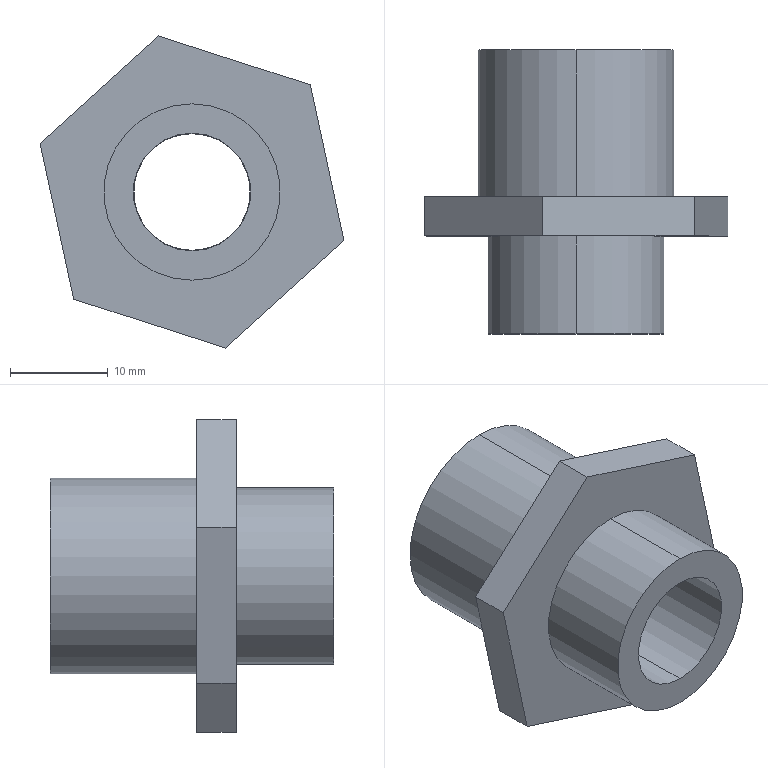Part | SolidWorks | features ICE 2, Extrusion 1 | 2 solids | 19 faces | box 31.039 x 29 x 31.865 mm | volume 6770 mm3 | plane 11 | cylinder 8 | commonest cylinder face diameters 11.911 x2 12 x2 18 x2 20 x2
STEP:
#1=CARTESIAN_POINT('',(0.,10.,-6.));
#2=VERTEX_POINT('',#1);
#3=CARTESIAN_POINT('',(0.,10.,6.));
#4=VERTEX_POINT('',#3);
#5=CARTESIAN_POINT('',(0.,10.,0.));
#6=DIRECTION('',(0.,1.,0.));
#7=DIRECTION('',(0.,0.,1.));
#8=AXIS2_PLACEMENT_3D('',#5,#6,#7);
#9=CIRCLE('',#8,6.);
#10=EDGE_CURVE('',#2,#4,#9,.T.);
#11=ORIENTED_EDGE('',*,*,#10,.T.);
#12=CARTESIAN_POINT('',(0.,0.,6.));
#13=VERTEX_POINT('',#12);
#14=CARTESIAN_POINT('',(0.,10.,6.));
#15=DIRECTION('',(0.,-1.,0.));
#16=VECTOR('',#15,1000.);
#17=LINE('',#14,#16);
#18=EDGE_CURVE('',#4,#13,#17,.T.);
#19=ORIENTED_EDGE('',*,*,#18,.T.);
#20=CARTESIAN_POINT('',(0.,0.,-6.));
#21=VERTEX_POINT('',#20);
#22=CARTESIAN_POINT('',(0.,0.,0.));
#23=DIRECTION('',(0.,1.,0.));
#24=DIRECTION('',(0.,0.,1.));
#25=AXIS2_PLACEMENT_3D('',#22,#23,#24);
#26=CIRCLE('',#25,6.);
#27=EDGE_CURVE('',#21,#13,#26,.T.);
#28=ORIENTED_EDGE('',*,*,#27,.F.);
#29=CARTESIAN_POINT('',(0.,10.,-6.));
#30=DIRECTION('',(0.,-1.,0.));
#31=VECTOR('',#30,1000.);
#32=LINE('',#29,#31);
#33=EDGE_CURVE('',#2,#21,#32,.T.);
#34=ORIENTED_EDGE('',*,*,#33,.F.);
#35=EDGE_LOOP('',(#11,#19,#28,#34));
#36=FACE_OUTER_BOUND('',#35,.T.);
#37=CARTESIAN_POINT('',(0.,10.,0.));
#38=DIRECTION('',(0.,-1.,0.));
#39=DIRECTION('',(0.,0.,-1.));
#40=AXIS2_PLACEMENT_3D('',#37,#38,#39);
#41=CYLINDRICAL_SURFACE('',#40,6.);
#42=ADVANCED_FACE('',(#36),#41,.F.);
#43=CARTESIAN_POINT('',(0.,10.,9.));
#44=VERTEX_POINT('',#43);
#45=CARTESIAN_POINT('',(0.,10.,-9.));
#46=VERTEX_POINT('',#45);
#47=CARTESIAN_POINT('',(0.,10.,0.));
#48=DIRECTION('',(0.,1.,0.));
#49=DIRECTION('',(0.,0.,1.));
#50=AXIS2_PLACEMENT_3D('',#47,#48,#49);
#51=CIRCLE('',#50,9.);
#52=EDGE_CURVE('',#44,#46,#51,.T.);
#53=ORIENTED_EDGE('',*,*,#52,.F.);
#54=CARTESIAN_POINT('',(0.,0.,9.));
#55=VERTEX_POINT('',#54);
#56=CARTESIAN_POINT('',(0.,10.,9.));
#57=DIRECTION('',(0.,-1.,0.));
#58=VECTOR('',#57,1000.);
#59=LINE('',#56,#58);
#60=EDGE_CURVE('',#44,#55,#59,.T.);
#61=ORIENTED_EDGE('',*,*,#60,.T.);
#62=CARTESIAN_POINT('',(0.,0.,-9.));
#63=VERTEX_POINT('',#62);
#64=CARTESIAN_POINT('',(0.,0.,0.));
#65=DIRECTION('',(0.,1.,0.));
#66=DIRECTION('',(0.,0.,1.));
#67=AXIS2_PLACEMENT_3D('',#64,#65,#66);
#68=CIRCLE('',#67,9.);
#69=EDGE_CURVE('',#55,#63,#68,.T.);
#70=ORIENTED_EDGE('',*,*,#69,.T.);
#71=CARTESIAN_POINT('',(0.,10.,-9.));
#72=DIRECTION('',(0.,-1.,0.));
#73=VECTOR('',#72,1000.);
#74=LINE('',#71,#73);
#75=EDGE_CURVE('',#46,#63,#74,.T.);
#76=ORIENTED_EDGE('',*,*,#75,.F.);
#77=EDGE_LOOP('',(#53,#61,#70,#76));
#78=FACE_OUTER_BOUND('',#77,.T.);
#79=CARTESIAN_POINT('',(0.,10.,0.));
#80=DIRECTION('',(0.,-1.,0.));
#81=DIRECTION('',(0.,0.,-1.));
#82=AXIS2_PLACEMENT_3D('',#79,#80,#81);
#83=CYLINDRICAL_SURFACE('',#82,9.);
#84=ADVANCED_FACE('',(#78),#83,.T.);
#85=CARTESIAN_POINT('',(0.,10.,0.));
#86=DIRECTION('',(0.,1.,0.));
#87=DIRECTION('',(0.,0.,1.));
#88=AXIS2_PLACEMENT_3D('',#85,#86,#87);
#89=CIRCLE('',#88,9.);
#90=EDGE_CURVE('',#46,#44,#89,.T.);
#91=ORIENTED_EDGE('',*,*,#90,.T.);
#92=ORIENTED_EDGE('',*,*,#52,.T.);
#93=EDGE_LOOP('',(#91,#92));
#94=FACE_OUTER_BOUND('',#93,.T.);
#95=ORIENTED_EDGE('',*,*,#10,.F.);
#96=CARTESIAN_POINT('',(0.,10.,0.));
#97=DIRECTION('',(0.,1.,0.));
#98=DIRECTION('',(0.,0.,1.));
#99=AXIS2_PLACEMENT_3D('',#96,#97,#98);
#100=CIRCLE('',#99,6.);
#101=EDGE_CURVE('',#4,#2,#100,.T.);
#102=ORIENTED_EDGE('',*,*,#101,.F.);
#103=EDGE_LOOP('',(#95,#102));
#104=FACE_BOUND('',#103,.T.);
#105=CARTESIAN_POINT('',(0.,10.,0.));
#106=DIRECTION('',(0.,1.,0.));
#107=DIRECTION('',(0.,0.,1.));
#108=AXIS2_PLACEMENT_3D('',#105,#106,#107);
#109=PLANE('',#108);
#110=ADVANCED_FACE('',(#94,#104),#109,.T.);
#111=CARTESIAN_POINT('',(0.,0.,0.));
#112=DIRECTION('',(0.,1.,0.));
#113=DIRECTION('',(0.,0.,1.));
#114=AXIS2_PLACEMENT_3D('',#111,#112,#113);
#115=CIRCLE('',#114,9.);
#116=EDGE_CURVE('',#63,#55,#115,.T.);
#117=ORIENTED_EDGE('',*,*,#116,.F.);
#118=ORIENTED_EDGE('',*,*,#69,.F.);
#119=EDGE_LOOP('',(#117,#118));
#120=FACE_OUTER_BOUND('',#119,.T.);
#121=ORIENTED_EDGE('',*,*,#27,.T.);
#122=CARTESIAN_POINT('',(0.,0.,0.));
#123=DIRECTION('',(0.,1.,0.));
#124=DIRECTION('',(0.,0.,1.));
#125=AXIS2_PLACEMENT_3D('',#122,#123,#124);
#126=CIRCLE('',#125,6.);
#127=EDGE_CURVE('',#13,#21,#126,.T.);
#128=ORIENTED_EDGE('',*,*,#127,.T.);
#129=EDGE_LOOP('',(#121,#128));
#130=FACE_BOUND('',#129,.T.);
#131=CARTESIAN_POINT('',(0.,0.,0.));
#132=DIRECTION('',(0.,1.,0.));
#133=DIRECTION('',(0.,0.,1.));
#134=AXIS2_PLACEMENT_3D('',#131,#132,#133);
#135=PLANE('',#134);
#136=ADVANCED_FACE('',(#120,#130),#135,.F.);
#137=ORIENTED_EDGE('',*,*,#60,.F.);
#138=ORIENTED_EDGE('',*,*,#90,.F.);
#139=ORIENTED_EDGE('',*,*,#75,.T.);
#140=ORIENTED_EDGE('',*,*,#116,.T.);
#141=EDGE_LOOP('',(#137,#138,#139,#140));
#142=FACE_OUTER_BOUND('',#141,.T.);
#143=CARTESIAN_POINT('',(0.,10.,0.));
#144=DIRECTION('',(0.,-1.,0.));
#145=DIRECTION('',(0.,0.,-1.));
#146=AXIS2_PLACEMENT_3D('',#143,#144,#145);
#147=CYLINDRICAL_SURFACE('',#146,9.);
#148=ADVANCED_FACE('',(#142),#147,.T.);
#149=ORIENTED_EDGE('',*,*,#18,.F.);
#150=ORIENTED_EDGE('',*,*,#101,.T.);
#151=ORIENTED_EDGE('',*,*,#33,.T.);
#152=ORIENTED_EDGE('',*,*,#127,.F.);
#153=EDGE_LOOP('',(#149,#150,#151,#152));
#154=FACE_OUTER_BOUND('',#153,.T.);
#155=CARTESIAN_POINT('',(0.,10.,0.));
#156=DIRECTION('',(0.,-1.,0.));
#157=DIRECTION('',(0.,0.,-1.));
#158=AXIS2_PLACEMENT_3D('',#155,#156,#157);
#159=CYLINDRICAL_SURFACE('',#158,6.);
#160=ADVANCED_FACE('',(#154),#159,.F.);
#161=CLOSED_SHELL('',(#42,#84,#110,#136,#148,#160));
#162=MANIFOLD_SOLID_BREP('',#161);
#163=CARTESIAN_POINT('',(0.,29.,10.));
#164=VERTEX_POINT('',#163);
#165=CARTESIAN_POINT('',(0.,29.,-10.));
#166=VERTEX_POINT('',#165);
#167=CARTESIAN_POINT('',(0.,29.,0.));
#168=DIRECTION('',(0.,1.,0.));
#169=DIRECTION('',(0.,0.,1.));
#170=AXIS2_PLACEMENT_3D('',#167,#168,#169);
#171=CIRCLE('',#170,10.);
#172=EDGE_CURVE('',#164,#166,#171,.T.);
#173=ORIENTED_EDGE('',*,*,#172,.F.);
#174=CARTESIAN_POINT('',(0.,14.,10.));
#175=VERTEX_POINT('',#174);
#176=CARTESIAN_POINT('',(0.,29.,10.));
#177=DIRECTION('',(0.,-1.,0.));
#178=VECTOR('',#177,1000.);
#179=LINE('',#176,#178);
#180=EDGE_CURVE('',#164,#175,#179,.T.);
#181=ORIENTED_EDGE('',*,*,#180,.T.);
#182=CARTESIAN_POINT('',(0.,14.,-10.));
#183=VERTEX_POINT('',#182);
#184=CARTESIAN_POINT('',(0.,14.,0.));
#185=DIRECTION('',(0.,1.,0.));
#186=DIRECTION('',(0.,0.,1.));
#187=AXIS2_PLACEMENT_3D('',#184,#185,#186);
#188=CIRCLE('',#187,10.);
#189=EDGE_CURVE('',#175,#183,#188,.T.);
#190=ORIENTED_EDGE('',*,*,#189,.T.);
#191=CARTESIAN_POINT('',(0.,29.,-10.));
#192=DIRECTION('',(0.,-1.,0.));
#193=VECTOR('',#192,1000.);
#194=LINE('',#191,#193);
#195=EDGE_CURVE('',#166,#183,#194,.T.);
#196=ORIENTED_EDGE('',*,*,#195,.F.);
#197=EDGE_LOOP('',(#173,#181,#190,#196));
#198=FACE_OUTER_BOUND('',#197,.T.);
#199=CARTESIAN_POINT('',(0.,29.,0.));
#200=DIRECTION('',(0.,-1.,0.));
#201=DIRECTION('',(0.,0.,-1.));
#202=AXIS2_PLACEMENT_3D('',#199,#200,#201);
#203=CYLINDRICAL_SURFACE('',#202,10.);
#204=ADVANCED_FACE('',(#198),#203,.T.);
#205=CARTESIAN_POINT('',(0.,29.,-5.955));
#206=VERTEX_POINT('',#205);
#207=CARTESIAN_POINT('',(0.,29.,5.955));
#208=VERTEX_POINT('',#207);
#209=CARTESIAN_POINT('',(0.,29.,0.));
#210=DIRECTION('',(0.,1.,0.));
#211=DIRECTION('',(0.,0.,1.));
#212=AXIS2_PLACEMENT_3D('',#209,#210,#211);
#213=CIRCLE('',#212,5.955);
#214=EDGE_CURVE('',#206,#208,#213,.T.);
#215=ORIENTED_EDGE('',*,*,#214,.T.);
#216=CARTESIAN_POINT('',(0.,10.,5.955));
#217=VERTEX_POINT('',#216);
#218=CARTESIAN_POINT('',(0.,14.,5.955));
#219=DIRECTION('',(0.,-1.,0.));
#220=VECTOR('',#219,1000.);
#221=LINE('',#218,#220);
#222=EDGE_CURVE('',#208,#217,#221,.T.);
#223=ORIENTED_EDGE('',*,*,#222,.T.);
#224=CARTESIAN_POINT('',(0.,10.,-5.955));
#225=VERTEX_POINT('',#224);
#226=CARTESIAN_POINT('',(0.,10.,0.));
#227=DIRECTION('',(0.,1.,0.));
#228=DIRECTION('',(0.,0.,1.));
#229=AXIS2_PLACEMENT_3D('',#226,#227,#228);
#230=CIRCLE('',#229,5.955);
#231=EDGE_CURVE('',#225,#217,#230,.T.);
#232=ORIENTED_EDGE('',*,*,#231,.F.);
#233=CARTESIAN_POINT('',(0.,14.,-5.955));
#234=DIRECTION('',(0.,-1.,0.));
#235=VECTOR('',#234,1000.);
#236=LINE('',#233,#235);
#237=EDGE_CURVE('',#206,#225,#236,.T.);
#238=ORIENTED_EDGE('',*,*,#237,.F.);
#239=EDGE_LOOP('',(#215,#223,#232,#238));
#240=FACE_OUTER_BOUND('',#239,.T.);
#241=CARTESIAN_POINT('',(0.,14.,0.));
#242=DIRECTION('',(0.,-1.,0.));
#243=DIRECTION('',(0.,0.,-1.));
#244=AXIS2_PLACEMENT_3D('',#241,#242,#243);
#245=CYLINDRICAL_SURFACE('',#244,5.955);
#246=ADVANCED_FACE('',(#240),#245,.F.);
#247=CARTESIAN_POINT('',(3.443,14.,-15.933));
#248=VERTEX_POINT('',#247);
#249=CARTESIAN_POINT('',(-12.076,14.,-10.948));
#250=VERTEX_POINT('',#249);
#251=CARTESIAN_POINT('',(3.443,14.,-15.933));
#252=DIRECTION('',(-0.9521,0.,0.3058));
#253=VECTOR('',#252,1000.);
#254=LINE('',#251,#253);
#255=EDGE_CURVE('',#248,#250,#254,.T.);
#256=ORIENTED_EDGE('',*,*,#255,.T.);
#257=CARTESIAN_POINT('',(-15.52,14.,4.984));
#258=VERTEX_POINT('',#257);
#259=CARTESIAN_POINT('',(-12.076,14.,-10.948));
#260=DIRECTION('',(-0.2112,0.,0.9774));
#261=VECTOR('',#260,1000.);
#262=LINE('',#259,#261);
#263=EDGE_CURVE('',#250,#258,#262,.T.);
#264=ORIENTED_EDGE('',*,*,#263,.T.);
#265=CARTESIAN_POINT('',(-3.443,14.,15.933));
#266=VERTEX_POINT('',#265);
#267=CARTESIAN_POINT('',(-15.52,14.,4.984));
#268=DIRECTION('',(0.7409,0.,0.6717));
#269=VECTOR('',#268,1000.);
#270=LINE('',#267,#269);
#271=EDGE_CURVE('',#258,#266,#270,.T.);
#272=ORIENTED_EDGE('',*,*,#271,.T.);
#273=CARTESIAN_POINT('',(12.076,14.,10.948));
#274=VERTEX_POINT('',#273);
#275=CARTESIAN_POINT('',(-3.443,14.,15.933));
#276=DIRECTION('',(0.9521,0.,-0.3058));
#277=VECTOR('',#276,1000.);
#278=LINE('',#275,#277);
#279=EDGE_CURVE('',#266,#274,#278,.T.);
#280=ORIENTED_EDGE('',*,*,#279,.T.);
#281=CARTESIAN_POINT('',(15.52,14.,-4.984));
#282=VERTEX_POINT('',#281);
#283=CARTESIAN_POINT('',(12.076,14.,10.948));
#284=DIRECTION('',(0.2112,0.,-0.9774));
#285=VECTOR('',#284,1000.);
#286=LINE('',#283,#285);
#287=EDGE_CURVE('',#274,#282,#286,.T.);
#288=ORIENTED_EDGE('',*,*,#287,.T.);
#289=CARTESIAN_POINT('',(15.52,14.,-4.984));
#290=DIRECTION('',(-0.7409,0.,-0.6717));
#291=VECTOR('',#290,1000.);
#292=LINE('',#289,#291);
#293=EDGE_CURVE('',#282,#248,#292,.T.);
#294=ORIENTED_EDGE('',*,*,#293,.T.);
#295=EDGE_LOOP('',(#256,#264,#272,#280,#288,#294));
#296=FACE_OUTER_BOUND('',#295,.T.);
#297=CARTESIAN_POINT('',(0.,14.,0.));
#298=DIRECTION('',(0.,1.,0.));
#299=DIRECTION('',(0.,0.,1.));
#300=AXIS2_PLACEMENT_3D('',#297,#298,#299);
#301=CIRCLE('',#300,10.);
#302=EDGE_CURVE('',#183,#175,#301,.T.);
#303=ORIENTED_EDGE('',*,*,#302,.F.);
#304=ORIENTED_EDGE('',*,*,#189,.F.);
#305=EDGE_LOOP('',(#303,#304));
#306=FACE_BOUND('',#305,.T.);
#307=CARTESIAN_POINT('',(0.,14.,0.));
#308=DIRECTION('',(0.,1.,0.));
#309=DIRECTION('',(0.,0.,1.));
#310=AXIS2_PLACEMENT_3D('',#307,#308,#309);
#311=PLANE('',#310);
#312=ADVANCED_FACE('',(#296,#306),#311,.T.);
#313=CARTESIAN_POINT('',(3.443,10.,-15.933));
#314=VERTEX_POINT('',#313);
#315=CARTESIAN_POINT('',(-12.076,10.,-10.948));
#316=VERTEX_POINT('',#315);
#317=CARTESIAN_POINT('',(3.443,10.,-15.933));
#318=DIRECTION('',(-0.9521,0.,0.3058));
#319=VECTOR('',#318,1000.);
#320=LINE('',#317,#319);
#321=EDGE_CURVE('',#314,#316,#320,.T.);
#322=ORIENTED_EDGE('',*,*,#321,.F.);
#323=CARTESIAN_POINT('',(15.52,10.,-4.984));
#324=VERTEX_POINT('',#323);
#325=CARTESIAN_POINT('',(15.52,10.,-4.984));
#326=DIRECTION('',(-0.7409,0.,-0.6717));
#327=VECTOR('',#326,1000.);
#328=LINE('',#325,#327);
#329=EDGE_CURVE('',#324,#314,#328,.T.);
#330=ORIENTED_EDGE('',*,*,#329,.F.);
#331=CARTESIAN_POINT('',(12.076,10.,10.948));
#332=VERTEX_POINT('',#331);
#333=CARTESIAN_POINT('',(12.076,10.,10.948));
#334=DIRECTION('',(0.2112,0.,-0.9774));
#335=VECTOR('',#334,1000.);
#336=LINE('',#333,#335);
#337=EDGE_CURVE('',#332,#324,#336,.T.);
#338=ORIENTED_EDGE('',*,*,#337,.F.);
#339=CARTESIAN_POINT('',(-3.443,10.,15.933));
#340=VERTEX_POINT('',#339);
#341=CARTESIAN_POINT('',(-3.443,10.,15.933));
#342=DIRECTION('',(0.9521,0.,-0.3058));
#343=VECTOR('',#342,1000.);
#344=LINE('',#341,#343);
#345=EDGE_CURVE('',#340,#332,#344,.T.);
#346=ORIENTED_EDGE('',*,*,#345,.F.);
#347=CARTESIAN_POINT('',(-15.52,10.,4.984));
#348=VERTEX_POINT('',#347);
#349=CARTESIAN_POINT('',(-15.52,10.,4.984));
#350=DIRECTION('',(0.7409,0.,0.6717));
#351=VECTOR('',#350,1000.);
#352=LINE('',#349,#351);
#353=EDGE_CURVE('',#348,#340,#352,.T.);
#354=ORIENTED_EDGE('',*,*,#353,.F.);
#355=CARTESIAN_POINT('',(-12.076,10.,-10.948));
#356=DIRECTION('',(-0.2112,0.,0.9774));
#357=VECTOR('',#356,1000.);
#358=LINE('',#355,#357);
#359=EDGE_CURVE('',#316,#348,#358,.T.);
#360=ORIENTED_EDGE('',*,*,#359,.F.);
#361=EDGE_LOOP('',(#322,#330,#338,#346,#354,#360));
#362=FACE_OUTER_BOUND('',#361,.T.);
#363=ORIENTED_EDGE('',*,*,#231,.T.);
#364=CARTESIAN_POINT('',(0.,10.,0.));
#365=DIRECTION('',(0.,1.,0.));
#366=DIRECTION('',(0.,0.,1.));
#367=AXIS2_PLACEMENT_3D('',#364,#365,#366);
#368=CIRCLE('',#367,5.955);
#369=EDGE_CURVE('',#217,#225,#368,.T.);
#370=ORIENTED_EDGE('',*,*,#369,.T.);
#371=EDGE_LOOP('',(#363,#370));
#372=FACE_BOUND('',#371,.T.);
#373=CARTESIAN_POINT('',(0.,10.,0.));
#374=DIRECTION('',(0.,1.,0.));
#375=DIRECTION('',(0.,0.,1.));
#376=AXIS2_PLACEMENT_3D('',#373,#374,#375);
#377=PLANE('',#376);
#378=ADVANCED_FACE('',(#362,#372),#377,.F.);
#379=ORIENTED_EDGE('',*,*,#321,.T.);
#380=CARTESIAN_POINT('',(-12.076,14.,-10.948));
#381=DIRECTION('',(0.,-1.,0.));
#382=VECTOR('',#381,1000.);
#383=LINE('',#380,#382);
#384=EDGE_CURVE('',#250,#316,#383,.T.);
#385=ORIENTED_EDGE('',*,*,#384,.F.);
#386=ORIENTED_EDGE('',*,*,#255,.F.);
#387=CARTESIAN_POINT('',(3.443,14.,-15.933));
#388=DIRECTION('',(0.,-1.,0.));
#389=VECTOR('',#388,1000.);
#390=LINE('',#387,#389);
#391=EDGE_CURVE('',#248,#314,#390,.T.);
#392=ORIENTED_EDGE('',*,*,#391,.T.);
#393=EDGE_LOOP('',(#379,#385,#386,#392));
#394=FACE_OUTER_BOUND('',#393,.T.);
#395=CARTESIAN_POINT('',(3.443,14.,-15.933));
#396=DIRECTION('',(0.3058,0.,0.9521));
#397=DIRECTION('',(0.9521,0.,-0.3058));
#398=AXIS2_PLACEMENT_3D('',#395,#396,#397);
#399=PLANE('',#398);
#400=ADVANCED_FACE('',(#394),#399,.F.);
#401=ORIENTED_EDGE('',*,*,#359,.T.);
#402=CARTESIAN_POINT('',(-15.52,14.,4.984));
#403=DIRECTION('',(0.,-1.,0.));
#404=VECTOR('',#403,1000.);
#405=LINE('',#402,#404);
#406=EDGE_CURVE('',#258,#348,#405,.T.);
#407=ORIENTED_EDGE('',*,*,#406,.F.);
#408=ORIENTED_EDGE('',*,*,#263,.F.);
#409=ORIENTED_EDGE('',*,*,#384,.T.);
#410=EDGE_LOOP('',(#401,#407,#408,#409));
#411=FACE_OUTER_BOUND('',#410,.T.);
#412=CARTESIAN_POINT('',(-12.076,14.,-10.948));
#413=DIRECTION('',(0.9774,0.,0.2112));
#414=DIRECTION('',(0.2112,0.,-0.9774));
#415=AXIS2_PLACEMENT_3D('',#412,#413,#414);
#416=PLANE('',#415);
#417=ADVANCED_FACE('',(#411),#416,.F.);
#418=ORIENTED_EDGE('',*,*,#353,.T.);
#419=CARTESIAN_POINT('',(-3.443,14.,15.933));
#420=DIRECTION('',(0.,-1.,0.));
#421=VECTOR('',#420,1000.);
#422=LINE('',#419,#421);
#423=EDGE_CURVE('',#266,#340,#422,.T.);
#424=ORIENTED_EDGE('',*,*,#423,.F.);
#425=ORIENTED_EDGE('',*,*,#271,.F.);
#426=ORIENTED_EDGE('',*,*,#406,.T.);
#427=EDGE_LOOP('',(#418,#424,#425,#426));
#428=FACE_OUTER_BOUND('',#427,.T.);
#429=CARTESIAN_POINT('',(-15.52,14.,4.984));
#430=DIRECTION('',(0.6717,0.,-0.7409));
#431=DIRECTION('',(-0.7409,0.,-0.6717));
#432=AXIS2_PLACEMENT_3D('',#429,#430,#431);
#433=PLANE('',#432);
#434=ADVANCED_FACE('',(#428),#433,.F.);
#435=ORIENTED_EDGE('',*,*,#345,.T.);
#436=CARTESIAN_POINT('',(12.076,14.,10.948));
#437=DIRECTION('',(0.,-1.,0.));
#438=VECTOR('',#437,1000.);
#439=LINE('',#436,#438);
#440=EDGE_CURVE('',#274,#332,#439,.T.);
#441=ORIENTED_EDGE('',*,*,#440,.F.);
#442=ORIENTED_EDGE('',*,*,#279,.F.);
#443=ORIENTED_EDGE('',*,*,#423,.T.);
#444=EDGE_LOOP('',(#435,#441,#442,#443));
#445=FACE_OUTER_BOUND('',#444,.T.);
#446=CARTESIAN_POINT('',(-3.443,14.,15.933));
#447=DIRECTION('',(-0.3058,0.,-0.9521));
#448=DIRECTION('',(-0.9521,0.,0.3058));
#449=AXIS2_PLACEMENT_3D('',#446,#447,#448);
#450=PLANE('',#449);
#451=ADVANCED_FACE('',(#445),#450,.F.);
#452=ORIENTED_EDGE('',*,*,#337,.T.);
#453=CARTESIAN_POINT('',(15.52,14.,-4.984));
#454=DIRECTION('',(0.,-1.,0.));
#455=VECTOR('',#454,1000.);
#456=LINE('',#453,#455);
#457=EDGE_CURVE('',#282,#324,#456,.T.);
#458=ORIENTED_EDGE('',*,*,#457,.F.);
#459=ORIENTED_EDGE('',*,*,#287,.F.);
#460=ORIENTED_EDGE('',*,*,#440,.T.);
#461=EDGE_LOOP('',(#452,#458,#459,#460));
#462=FACE_OUTER_BOUND('',#461,.T.);
#463=CARTESIAN_POINT('',(12.076,14.,10.948));
#464=DIRECTION('',(-0.9774,0.,-0.2112));
#465=DIRECTION('',(-0.2112,0.,0.9774));
#466=AXIS2_PLACEMENT_3D('',#463,#464,#465);
#467=PLANE('',#466);
#468=ADVANCED_FACE('',(#462),#467,.F.);
#469=ORIENTED_EDGE('',*,*,#329,.T.);
#470=ORIENTED_EDGE('',*,*,#391,.F.);
#471=ORIENTED_EDGE('',*,*,#293,.F.);
#472=ORIENTED_EDGE('',*,*,#457,.T.);
#473=EDGE_LOOP('',(#469,#470,#471,#472));
#474=FACE_OUTER_BOUND('',#473,.T.);
#475=CARTESIAN_POINT('',(15.52,14.,-4.984));
#476=DIRECTION('',(-0.6717,0.,0.7409));
#477=DIRECTION('',(0.7409,0.,0.6717));
#478=AXIS2_PLACEMENT_3D('',#475,#476,#477);
#479=PLANE('',#478);
#480=ADVANCED_FACE('',(#474),#479,.F.);
#481=ORIENTED_EDGE('',*,*,#222,.F.);
#482=CARTESIAN_POINT('',(0.,29.,0.));
#483=DIRECTION('',(0.,1.,0.));
#484=DIRECTION('',(0.,0.,1.));
#485=AXIS2_PLACEMENT_3D('',#482,#483,#484);
#486=CIRCLE('',#485,5.955);
#487=EDGE_CURVE('',#208,#206,#486,.T.);
#488=ORIENTED_EDGE('',*,*,#487,.T.);
#489=ORIENTED_EDGE('',*,*,#237,.T.);
#490=ORIENTED_EDGE('',*,*,#369,.F.);
#491=EDGE_LOOP('',(#481,#488,#489,#490));
#492=FACE_OUTER_BOUND('',#491,.T.);
#493=CARTESIAN_POINT('',(0.,14.,0.));
#494=DIRECTION('',(0.,-1.,0.));
#495=DIRECTION('',(0.,0.,-1.));
#496=AXIS2_PLACEMENT_3D('',#493,#494,#495);
#497=CYLINDRICAL_SURFACE('',#496,5.955);
#498=ADVANCED_FACE('',(#492),#497,.F.);
#499=CARTESIAN_POINT('',(0.,29.,0.));
#500=DIRECTION('',(0.,1.,0.));
#501=DIRECTION('',(0.,0.,1.));
#502=AXIS2_PLACEMENT_3D('',#499,#500,#501);
#503=CIRCLE('',#502,10.);
#504=EDGE_CURVE('',#166,#164,#503,.T.);
#505=ORIENTED_EDGE('',*,*,#504,.T.);
#506=ORIENTED_EDGE('',*,*,#172,.T.);
#507=EDGE_LOOP('',(#505,#506));
#508=FACE_OUTER_BOUND('',#507,.T.);
#509=ORIENTED_EDGE('',*,*,#214,.F.);
#510=ORIENTED_EDGE('',*,*,#487,.F.);
#511=EDGE_LOOP('',(#509,#510));
#512=FACE_BOUND('',#511,.T.);
#513=CARTESIAN_POINT('',(0.,29.,0.));
#514=DIRECTION('',(0.,1.,0.));
#515=DIRECTION('',(0.,0.,1.));
#516=AXIS2_PLACEMENT_3D('',#513,#514,#515);
#517=PLANE('',#516);
#518=ADVANCED_FACE('',(#508,#512),#517,.T.);
#519=ORIENTED_EDGE('',*,*,#180,.F.);
#520=ORIENTED_EDGE('',*,*,#504,.F.);
#521=ORIENTED_EDGE('',*,*,#195,.T.);
#522=ORIENTED_EDGE('',*,*,#302,.T.);
#523=EDGE_LOOP('',(#519,#520,#521,#522));
#524=FACE_OUTER_BOUND('',#523,.T.);
#525=CARTESIAN_POINT('',(0.,29.,0.));
#526=DIRECTION('',(0.,-1.,0.));
#527=DIRECTION('',(0.,0.,-1.));
#528=AXIS2_PLACEMENT_3D('',#525,#526,#527);
#529=CYLINDRICAL_SURFACE('',#528,10.);
#530=ADVANCED_FACE('',(#524),#529,.T.);
#531=CLOSED_SHELL('',(#204,#246,#312,#378,#400,#417,#434,#451,#468,#480,#498,#518,#530));
#532=MANIFOLD_SOLID_BREP('',#531);
#533=CARTESIAN_POINT('',(0.,0.,0.));
#534=DIRECTION('',(0.,0.,1.));
#535=DIRECTION('',(1.,0.,0.));
#536=AXIS2_PLACEMENT_3D('',#533,#534,#535);
#537=(LENGTH_UNIT()NAMED_UNIT(*)SI_UNIT(.MILLI.,.METRE.));
#538=UNCERTAINTY_MEASURE_WITH_UNIT(LENGTH_MEASURE(0.00001),#537,'','');
#539=(NAMED_UNIT(*)PLANE_ANGLE_UNIT()SI_UNIT($,.RADIAN.));
#540=(NAMED_UNIT(*)SI_UNIT($,.STERADIAN.)SOLID_ANGLE_UNIT());
#541=(GEOMETRIC_REPRESENTATION_CONTEXT(3)GLOBAL_UNCERTAINTY_ASSIGNED_CONTEXT((#538))GLOBAL_UNIT_ASSIGNED_CONTEXT((#537,#539,#540))REPRESENTATION_CONTEXT('',''));
#542=ADVANCED_BREP_SHAPE_REPRESENTATION('',(#162,#532,#536),#541);